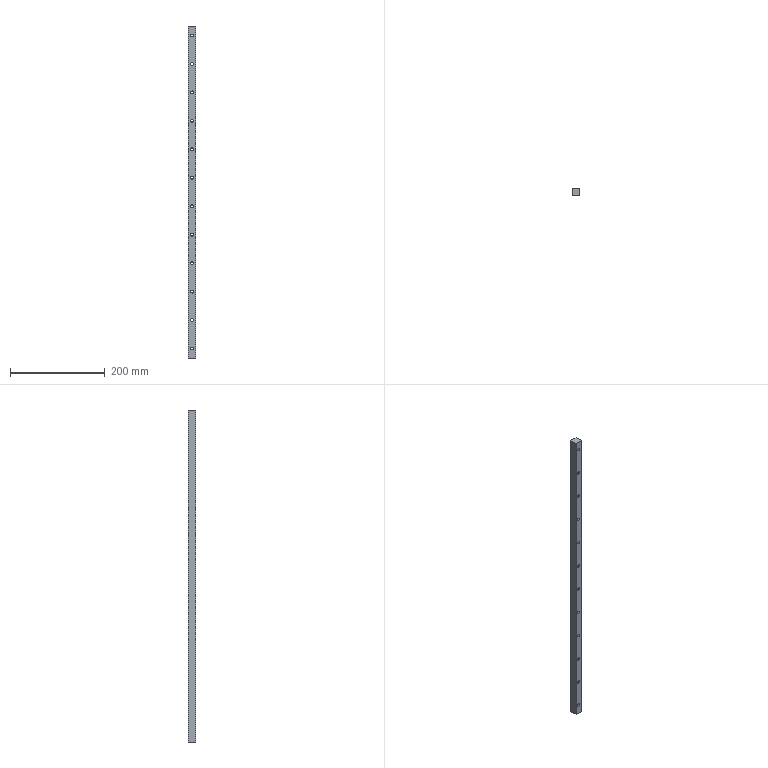Part | 1 solid | 30 faces | box 15 x 15 x 700 mm | volume 152411 mm3 | cylinder 24 | plane 6 | commonest cylinder face diameters 6 x24
STEP:
#1=CARTESIAN_POINT('',(7.5,0.,677.));
#2=VERTEX_POINT('',#1);
#3=CARTESIAN_POINT('',(7.5,0.,683.));
#4=VERTEX_POINT('',#3);
#5=CARTESIAN_POINT('',(7.5,0.,680.));
#6=DIRECTION('',(0.,1.,0.));
#7=DIRECTION('',(0.,0.,1.));
#8=AXIS2_PLACEMENT_3D('',#5,#6,#7);
#9=CIRCLE('',#8,3.);
#10=EDGE_CURVE('',#2,#4,#9,.T.);
#11=ORIENTED_EDGE('',*,*,#10,.F.);
#12=CARTESIAN_POINT('',(7.5,15.,677.));
#13=VERTEX_POINT('',#12);
#14=CARTESIAN_POINT('',(7.5,-35.,677.));
#15=DIRECTION('',(0.,1.,0.));
#16=VECTOR('',#15,1000.);
#17=LINE('',#14,#16);
#18=EDGE_CURVE('',#2,#13,#17,.T.);
#19=ORIENTED_EDGE('',*,*,#18,.T.);
#20=CARTESIAN_POINT('',(7.5,15.,683.));
#21=VERTEX_POINT('',#20);
#22=CARTESIAN_POINT('',(7.5,15.,680.));
#23=DIRECTION('',(0.,1.,0.));
#24=DIRECTION('',(0.,0.,1.));
#25=AXIS2_PLACEMENT_3D('',#22,#23,#24);
#26=CIRCLE('',#25,3.);
#27=EDGE_CURVE('',#13,#21,#26,.T.);
#28=ORIENTED_EDGE('',*,*,#27,.T.);
#29=CARTESIAN_POINT('',(7.5,-35.,683.));
#30=DIRECTION('',(0.,1.,0.));
#31=VECTOR('',#30,1000.);
#32=LINE('',#29,#31);
#33=EDGE_CURVE('',#4,#21,#32,.T.);
#34=ORIENTED_EDGE('',*,*,#33,.F.);
#35=EDGE_LOOP('',(#11,#19,#28,#34));
#36=FACE_OUTER_BOUND('',#35,.T.);
#37=CARTESIAN_POINT('',(7.5,-35.,680.));
#38=DIRECTION('',(0.,1.,0.));
#39=DIRECTION('',(0.,0.,1.));
#40=AXIS2_PLACEMENT_3D('',#37,#38,#39);
#41=CYLINDRICAL_SURFACE('',#40,3.);
#42=ADVANCED_FACE('',(#36),#41,.F.);
#43=CARTESIAN_POINT('',(7.5,0.,617.));
#44=VERTEX_POINT('',#43);
#45=CARTESIAN_POINT('',(7.5,0.,623.));
#46=VERTEX_POINT('',#45);
#47=CARTESIAN_POINT('',(7.5,0.,620.));
#48=DIRECTION('',(0.,1.,0.));
#49=DIRECTION('',(0.,0.,1.));
#50=AXIS2_PLACEMENT_3D('',#47,#48,#49);
#51=CIRCLE('',#50,3.);
#52=EDGE_CURVE('',#44,#46,#51,.T.);
#53=ORIENTED_EDGE('',*,*,#52,.F.);
#54=CARTESIAN_POINT('',(7.5,15.,617.));
#55=VERTEX_POINT('',#54);
#56=CARTESIAN_POINT('',(7.5,-35.,617.));
#57=DIRECTION('',(0.,1.,0.));
#58=VECTOR('',#57,1000.);
#59=LINE('',#56,#58);
#60=EDGE_CURVE('',#44,#55,#59,.T.);
#61=ORIENTED_EDGE('',*,*,#60,.T.);
#62=CARTESIAN_POINT('',(7.5,15.,623.));
#63=VERTEX_POINT('',#62);
#64=CARTESIAN_POINT('',(7.5,15.,620.));
#65=DIRECTION('',(0.,1.,0.));
#66=DIRECTION('',(0.,0.,1.));
#67=AXIS2_PLACEMENT_3D('',#64,#65,#66);
#68=CIRCLE('',#67,3.);
#69=EDGE_CURVE('',#55,#63,#68,.T.);
#70=ORIENTED_EDGE('',*,*,#69,.T.);
#71=CARTESIAN_POINT('',(7.5,-35.,623.));
#72=DIRECTION('',(0.,1.,0.));
#73=VECTOR('',#72,1000.);
#74=LINE('',#71,#73);
#75=EDGE_CURVE('',#46,#63,#74,.T.);
#76=ORIENTED_EDGE('',*,*,#75,.F.);
#77=EDGE_LOOP('',(#53,#61,#70,#76));
#78=FACE_OUTER_BOUND('',#77,.T.);
#79=CARTESIAN_POINT('',(7.5,-35.,620.));
#80=DIRECTION('',(0.,1.,0.));
#81=DIRECTION('',(0.,0.,1.));
#82=AXIS2_PLACEMENT_3D('',#79,#80,#81);
#83=CYLINDRICAL_SURFACE('',#82,3.);
#84=ADVANCED_FACE('',(#78),#83,.F.);
#85=CARTESIAN_POINT('',(7.5,0.,557.));
#86=VERTEX_POINT('',#85);
#87=CARTESIAN_POINT('',(7.5,0.,563.));
#88=VERTEX_POINT('',#87);
#89=CARTESIAN_POINT('',(7.5,0.,560.));
#90=DIRECTION('',(0.,1.,0.));
#91=DIRECTION('',(0.,0.,1.));
#92=AXIS2_PLACEMENT_3D('',#89,#90,#91);
#93=CIRCLE('',#92,3.);
#94=EDGE_CURVE('',#86,#88,#93,.T.);
#95=ORIENTED_EDGE('',*,*,#94,.F.);
#96=CARTESIAN_POINT('',(7.5,15.,557.));
#97=VERTEX_POINT('',#96);
#98=CARTESIAN_POINT('',(7.5,-35.,557.));
#99=DIRECTION('',(0.,1.,0.));
#100=VECTOR('',#99,1000.);
#101=LINE('',#98,#100);
#102=EDGE_CURVE('',#86,#97,#101,.T.);
#103=ORIENTED_EDGE('',*,*,#102,.T.);
#104=CARTESIAN_POINT('',(7.5,15.,563.));
#105=VERTEX_POINT('',#104);
#106=CARTESIAN_POINT('',(7.5,15.,560.));
#107=DIRECTION('',(0.,1.,0.));
#108=DIRECTION('',(0.,0.,1.));
#109=AXIS2_PLACEMENT_3D('',#106,#107,#108);
#110=CIRCLE('',#109,3.);
#111=EDGE_CURVE('',#97,#105,#110,.T.);
#112=ORIENTED_EDGE('',*,*,#111,.T.);
#113=CARTESIAN_POINT('',(7.5,-35.,563.));
#114=DIRECTION('',(0.,1.,0.));
#115=VECTOR('',#114,1000.);
#116=LINE('',#113,#115);
#117=EDGE_CURVE('',#88,#105,#116,.T.);
#118=ORIENTED_EDGE('',*,*,#117,.F.);
#119=EDGE_LOOP('',(#95,#103,#112,#118));
#120=FACE_OUTER_BOUND('',#119,.T.);
#121=CARTESIAN_POINT('',(7.5,-35.,560.));
#122=DIRECTION('',(0.,1.,0.));
#123=DIRECTION('',(0.,0.,1.));
#124=AXIS2_PLACEMENT_3D('',#121,#122,#123);
#125=CYLINDRICAL_SURFACE('',#124,3.);
#126=ADVANCED_FACE('',(#120),#125,.F.);
#127=CARTESIAN_POINT('',(7.5,0.,497.));
#128=VERTEX_POINT('',#127);
#129=CARTESIAN_POINT('',(7.5,0.,503.));
#130=VERTEX_POINT('',#129);
#131=CARTESIAN_POINT('',(7.5,0.,500.));
#132=DIRECTION('',(0.,1.,0.));
#133=DIRECTION('',(0.,0.,1.));
#134=AXIS2_PLACEMENT_3D('',#131,#132,#133);
#135=CIRCLE('',#134,3.);
#136=EDGE_CURVE('',#128,#130,#135,.T.);
#137=ORIENTED_EDGE('',*,*,#136,.F.);
#138=CARTESIAN_POINT('',(7.5,15.,497.));
#139=VERTEX_POINT('',#138);
#140=CARTESIAN_POINT('',(7.5,-35.,497.));
#141=DIRECTION('',(0.,1.,0.));
#142=VECTOR('',#141,1000.);
#143=LINE('',#140,#142);
#144=EDGE_CURVE('',#128,#139,#143,.T.);
#145=ORIENTED_EDGE('',*,*,#144,.T.);
#146=CARTESIAN_POINT('',(7.5,15.,503.));
#147=VERTEX_POINT('',#146);
#148=CARTESIAN_POINT('',(7.5,15.,500.));
#149=DIRECTION('',(0.,1.,0.));
#150=DIRECTION('',(0.,0.,1.));
#151=AXIS2_PLACEMENT_3D('',#148,#149,#150);
#152=CIRCLE('',#151,3.);
#153=EDGE_CURVE('',#139,#147,#152,.T.);
#154=ORIENTED_EDGE('',*,*,#153,.T.);
#155=CARTESIAN_POINT('',(7.5,-35.,503.));
#156=DIRECTION('',(0.,1.,0.));
#157=VECTOR('',#156,1000.);
#158=LINE('',#155,#157);
#159=EDGE_CURVE('',#130,#147,#158,.T.);
#160=ORIENTED_EDGE('',*,*,#159,.F.);
#161=EDGE_LOOP('',(#137,#145,#154,#160));
#162=FACE_OUTER_BOUND('',#161,.T.);
#163=CARTESIAN_POINT('',(7.5,-35.,500.));
#164=DIRECTION('',(0.,1.,0.));
#165=DIRECTION('',(0.,0.,1.));
#166=AXIS2_PLACEMENT_3D('',#163,#164,#165);
#167=CYLINDRICAL_SURFACE('',#166,3.);
#168=ADVANCED_FACE('',(#162),#167,.F.);
#169=CARTESIAN_POINT('',(7.5,0.,437.));
#170=VERTEX_POINT('',#169);
#171=CARTESIAN_POINT('',(7.5,0.,443.));
#172=VERTEX_POINT('',#171);
#173=CARTESIAN_POINT('',(7.5,0.,440.));
#174=DIRECTION('',(0.,1.,0.));
#175=DIRECTION('',(0.,0.,1.));
#176=AXIS2_PLACEMENT_3D('',#173,#174,#175);
#177=CIRCLE('',#176,3.);
#178=EDGE_CURVE('',#170,#172,#177,.T.);
#179=ORIENTED_EDGE('',*,*,#178,.F.);
#180=CARTESIAN_POINT('',(7.5,15.,437.));
#181=VERTEX_POINT('',#180);
#182=CARTESIAN_POINT('',(7.5,-35.,437.));
#183=DIRECTION('',(0.,1.,0.));
#184=VECTOR('',#183,1000.);
#185=LINE('',#182,#184);
#186=EDGE_CURVE('',#170,#181,#185,.T.);
#187=ORIENTED_EDGE('',*,*,#186,.T.);
#188=CARTESIAN_POINT('',(7.5,15.,443.));
#189=VERTEX_POINT('',#188);
#190=CARTESIAN_POINT('',(7.5,15.,440.));
#191=DIRECTION('',(0.,1.,0.));
#192=DIRECTION('',(0.,0.,1.));
#193=AXIS2_PLACEMENT_3D('',#190,#191,#192);
#194=CIRCLE('',#193,3.);
#195=EDGE_CURVE('',#181,#189,#194,.T.);
#196=ORIENTED_EDGE('',*,*,#195,.T.);
#197=CARTESIAN_POINT('',(7.5,-35.,443.));
#198=DIRECTION('',(0.,1.,0.));
#199=VECTOR('',#198,1000.);
#200=LINE('',#197,#199);
#201=EDGE_CURVE('',#172,#189,#200,.T.);
#202=ORIENTED_EDGE('',*,*,#201,.F.);
#203=EDGE_LOOP('',(#179,#187,#196,#202));
#204=FACE_OUTER_BOUND('',#203,.T.);
#205=CARTESIAN_POINT('',(7.5,-35.,440.));
#206=DIRECTION('',(0.,1.,0.));
#207=DIRECTION('',(0.,0.,1.));
#208=AXIS2_PLACEMENT_3D('',#205,#206,#207);
#209=CYLINDRICAL_SURFACE('',#208,3.);
#210=ADVANCED_FACE('',(#204),#209,.F.);
#211=CARTESIAN_POINT('',(7.5,0.,377.));
#212=VERTEX_POINT('',#211);
#213=CARTESIAN_POINT('',(7.5,0.,383.));
#214=VERTEX_POINT('',#213);
#215=CARTESIAN_POINT('',(7.5,0.,380.));
#216=DIRECTION('',(0.,1.,0.));
#217=DIRECTION('',(0.,0.,1.));
#218=AXIS2_PLACEMENT_3D('',#215,#216,#217);
#219=CIRCLE('',#218,3.);
#220=EDGE_CURVE('',#212,#214,#219,.T.);
#221=ORIENTED_EDGE('',*,*,#220,.F.);
#222=CARTESIAN_POINT('',(7.5,15.,377.));
#223=VERTEX_POINT('',#222);
#224=CARTESIAN_POINT('',(7.5,-35.,377.));
#225=DIRECTION('',(0.,1.,0.));
#226=VECTOR('',#225,1000.);
#227=LINE('',#224,#226);
#228=EDGE_CURVE('',#212,#223,#227,.T.);
#229=ORIENTED_EDGE('',*,*,#228,.T.);
#230=CARTESIAN_POINT('',(7.5,15.,383.));
#231=VERTEX_POINT('',#230);
#232=CARTESIAN_POINT('',(7.5,15.,380.));
#233=DIRECTION('',(0.,1.,0.));
#234=DIRECTION('',(0.,0.,1.));
#235=AXIS2_PLACEMENT_3D('',#232,#233,#234);
#236=CIRCLE('',#235,3.);
#237=EDGE_CURVE('',#223,#231,#236,.T.);
#238=ORIENTED_EDGE('',*,*,#237,.T.);
#239=CARTESIAN_POINT('',(7.5,-35.,383.));
#240=DIRECTION('',(0.,1.,0.));
#241=VECTOR('',#240,1000.);
#242=LINE('',#239,#241);
#243=EDGE_CURVE('',#214,#231,#242,.T.);
#244=ORIENTED_EDGE('',*,*,#243,.F.);
#245=EDGE_LOOP('',(#221,#229,#238,#244));
#246=FACE_OUTER_BOUND('',#245,.T.);
#247=CARTESIAN_POINT('',(7.5,-35.,380.));
#248=DIRECTION('',(0.,1.,0.));
#249=DIRECTION('',(0.,0.,1.));
#250=AXIS2_PLACEMENT_3D('',#247,#248,#249);
#251=CYLINDRICAL_SURFACE('',#250,3.);
#252=ADVANCED_FACE('',(#246),#251,.F.);
#253=CARTESIAN_POINT('',(7.5,0.,317.));
#254=VERTEX_POINT('',#253);
#255=CARTESIAN_POINT('',(7.5,0.,323.));
#256=VERTEX_POINT('',#255);
#257=CARTESIAN_POINT('',(7.5,0.,320.));
#258=DIRECTION('',(0.,1.,0.));
#259=DIRECTION('',(0.,0.,1.));
#260=AXIS2_PLACEMENT_3D('',#257,#258,#259);
#261=CIRCLE('',#260,3.);
#262=EDGE_CURVE('',#254,#256,#261,.T.);
#263=ORIENTED_EDGE('',*,*,#262,.F.);
#264=CARTESIAN_POINT('',(7.5,15.,317.));
#265=VERTEX_POINT('',#264);
#266=CARTESIAN_POINT('',(7.5,-35.,317.));
#267=DIRECTION('',(0.,1.,0.));
#268=VECTOR('',#267,1000.);
#269=LINE('',#266,#268);
#270=EDGE_CURVE('',#254,#265,#269,.T.);
#271=ORIENTED_EDGE('',*,*,#270,.T.);
#272=CARTESIAN_POINT('',(7.5,15.,323.));
#273=VERTEX_POINT('',#272);
#274=CARTESIAN_POINT('',(7.5,15.,320.));
#275=DIRECTION('',(0.,1.,0.));
#276=DIRECTION('',(0.,0.,1.));
#277=AXIS2_PLACEMENT_3D('',#274,#275,#276);
#278=CIRCLE('',#277,3.);
#279=EDGE_CURVE('',#265,#273,#278,.T.);
#280=ORIENTED_EDGE('',*,*,#279,.T.);
#281=CARTESIAN_POINT('',(7.5,-35.,323.));
#282=DIRECTION('',(0.,1.,0.));
#283=VECTOR('',#282,1000.);
#284=LINE('',#281,#283);
#285=EDGE_CURVE('',#256,#273,#284,.T.);
#286=ORIENTED_EDGE('',*,*,#285,.F.);
#287=EDGE_LOOP('',(#263,#271,#280,#286));
#288=FACE_OUTER_BOUND('',#287,.T.);
#289=CARTESIAN_POINT('',(7.5,-35.,320.));
#290=DIRECTION('',(0.,1.,0.));
#291=DIRECTION('',(0.,0.,1.));
#292=AXIS2_PLACEMENT_3D('',#289,#290,#291);
#293=CYLINDRICAL_SURFACE('',#292,3.);
#294=ADVANCED_FACE('',(#288),#293,.F.);
#295=CARTESIAN_POINT('',(7.5,0.,257.));
#296=VERTEX_POINT('',#295);
#297=CARTESIAN_POINT('',(7.5,0.,263.));
#298=VERTEX_POINT('',#297);
#299=CARTESIAN_POINT('',(7.5,0.,260.));
#300=DIRECTION('',(0.,1.,0.));
#301=DIRECTION('',(0.,0.,1.));
#302=AXIS2_PLACEMENT_3D('',#299,#300,#301);
#303=CIRCLE('',#302,3.);
#304=EDGE_CURVE('',#296,#298,#303,.T.);
#305=ORIENTED_EDGE('',*,*,#304,.F.);
#306=CARTESIAN_POINT('',(7.5,15.,257.));
#307=VERTEX_POINT('',#306);
#308=CARTESIAN_POINT('',(7.5,-35.,257.));
#309=DIRECTION('',(0.,1.,0.));
#310=VECTOR('',#309,1000.);
#311=LINE('',#308,#310);
#312=EDGE_CURVE('',#296,#307,#311,.T.);
#313=ORIENTED_EDGE('',*,*,#312,.T.);
#314=CARTESIAN_POINT('',(7.5,15.,263.));
#315=VERTEX_POINT('',#314);
#316=CARTESIAN_POINT('',(7.5,15.,260.));
#317=DIRECTION('',(0.,1.,0.));
#318=DIRECTION('',(0.,0.,1.));
#319=AXIS2_PLACEMENT_3D('',#316,#317,#318);
#320=CIRCLE('',#319,3.);
#321=EDGE_CURVE('',#307,#315,#320,.T.);
#322=ORIENTED_EDGE('',*,*,#321,.T.);
#323=CARTESIAN_POINT('',(7.5,-35.,263.));
#324=DIRECTION('',(0.,1.,0.));
#325=VECTOR('',#324,1000.);
#326=LINE('',#323,#325);
#327=EDGE_CURVE('',#298,#315,#326,.T.);
#328=ORIENTED_EDGE('',*,*,#327,.F.);
#329=EDGE_LOOP('',(#305,#313,#322,#328));
#330=FACE_OUTER_BOUND('',#329,.T.);
#331=CARTESIAN_POINT('',(7.5,-35.,260.));
#332=DIRECTION('',(0.,1.,0.));
#333=DIRECTION('',(0.,0.,1.));
#334=AXIS2_PLACEMENT_3D('',#331,#332,#333);
#335=CYLINDRICAL_SURFACE('',#334,3.);
#336=ADVANCED_FACE('',(#330),#335,.F.);
#337=CARTESIAN_POINT('',(7.5,0.,197.));
#338=VERTEX_POINT('',#337);
#339=CARTESIAN_POINT('',(7.5,0.,203.));
#340=VERTEX_POINT('',#339);
#341=CARTESIAN_POINT('',(7.5,0.,200.));
#342=DIRECTION('',(0.,1.,0.));
#343=DIRECTION('',(0.,0.,1.));
#344=AXIS2_PLACEMENT_3D('',#341,#342,#343);
#345=CIRCLE('',#344,3.);
#346=EDGE_CURVE('',#338,#340,#345,.T.);
#347=ORIENTED_EDGE('',*,*,#346,.F.);
#348=CARTESIAN_POINT('',(7.5,15.,197.));
#349=VERTEX_POINT('',#348);
#350=CARTESIAN_POINT('',(7.5,-35.,197.));
#351=DIRECTION('',(0.,1.,0.));
#352=VECTOR('',#351,1000.);
#353=LINE('',#350,#352);
#354=EDGE_CURVE('',#338,#349,#353,.T.);
#355=ORIENTED_EDGE('',*,*,#354,.T.);
#356=CARTESIAN_POINT('',(7.5,15.,203.));
#357=VERTEX_POINT('',#356);
#358=CARTESIAN_POINT('',(7.5,15.,200.));
#359=DIRECTION('',(0.,1.,0.));
#360=DIRECTION('',(0.,0.,1.));
#361=AXIS2_PLACEMENT_3D('',#358,#359,#360);
#362=CIRCLE('',#361,3.);
#363=EDGE_CURVE('',#349,#357,#362,.T.);
#364=ORIENTED_EDGE('',*,*,#363,.T.);
#365=CARTESIAN_POINT('',(7.5,-35.,203.));
#366=DIRECTION('',(0.,1.,0.));
#367=VECTOR('',#366,1000.);
#368=LINE('',#365,#367);
#369=EDGE_CURVE('',#340,#357,#368,.T.);
#370=ORIENTED_EDGE('',*,*,#369,.F.);
#371=EDGE_LOOP('',(#347,#355,#364,#370));
#372=FACE_OUTER_BOUND('',#371,.T.);
#373=CARTESIAN_POINT('',(7.5,-35.,200.));
#374=DIRECTION('',(0.,1.,0.));
#375=DIRECTION('',(0.,0.,1.));
#376=AXIS2_PLACEMENT_3D('',#373,#374,#375);
#377=CYLINDRICAL_SURFACE('',#376,3.);
#378=ADVANCED_FACE('',(#372),#377,.F.);
#379=CARTESIAN_POINT('',(7.5,0.,137.));
#380=VERTEX_POINT('',#379);
#381=CARTESIAN_POINT('',(7.5,0.,143.));
#382=VERTEX_POINT('',#381);
#383=CARTESIAN_POINT('',(7.5,0.,140.));
#384=DIRECTION('',(0.,1.,0.));
#385=DIRECTION('',(0.,0.,1.));
#386=AXIS2_PLACEMENT_3D('',#383,#384,#385);
#387=CIRCLE('',#386,3.);
#388=EDGE_CURVE('',#380,#382,#387,.T.);
#389=ORIENTED_EDGE('',*,*,#388,.F.);
#390=CARTESIAN_POINT('',(7.5,15.,137.));
#391=VERTEX_POINT('',#390);
#392=CARTESIAN_POINT('',(7.5,-35.,137.));
#393=DIRECTION('',(0.,1.,0.));
#394=VECTOR('',#393,1000.);
#395=LINE('',#392,#394);
#396=EDGE_CURVE('',#380,#391,#395,.T.);
#397=ORIENTED_EDGE('',*,*,#396,.T.);
#398=CARTESIAN_POINT('',(7.5,15.,143.));
#399=VERTEX_POINT('',#398);
#400=CARTESIAN_POINT('',(7.5,15.,140.));
#401=DIRECTION('',(0.,1.,0.));
#402=DIRECTION('',(0.,0.,1.));
#403=AXIS2_PLACEMENT_3D('',#400,#401,#402);
#404=CIRCLE('',#403,3.);
#405=EDGE_CURVE('',#391,#399,#404,.T.);
#406=ORIENTED_EDGE('',*,*,#405,.T.);
#407=CARTESIAN_POINT('',(7.5,-35.,143.));
#408=DIRECTION('',(0.,1.,0.));
#409=VECTOR('',#408,1000.);
#410=LINE('',#407,#409);
#411=EDGE_CURVE('',#382,#399,#410,.T.);
#412=ORIENTED_EDGE('',*,*,#411,.F.);
#413=EDGE_LOOP('',(#389,#397,#406,#412));
#414=FACE_OUTER_BOUND('',#413,.T.);
#415=CARTESIAN_POINT('',(7.5,-35.,140.));
#416=DIRECTION('',(0.,1.,0.));
#417=DIRECTION('',(0.,0.,1.));
#418=AXIS2_PLACEMENT_3D('',#415,#416,#417);
#419=CYLINDRICAL_SURFACE('',#418,3.);
#420=ADVANCED_FACE('',(#414),#419,.F.);
#421=CARTESIAN_POINT('',(7.5,0.,77.));
#422=VERTEX_POINT('',#421);
#423=CARTESIAN_POINT('',(7.5,0.,83.));
#424=VERTEX_POINT('',#423);
#425=CARTESIAN_POINT('',(7.5,0.,80.));
#426=DIRECTION('',(0.,1.,0.));
#427=DIRECTION('',(0.,0.,1.));
#428=AXIS2_PLACEMENT_3D('',#425,#426,#427);
#429=CIRCLE('',#428,3.);
#430=EDGE_CURVE('',#422,#424,#429,.T.);
#431=ORIENTED_EDGE('',*,*,#430,.F.);
#432=CARTESIAN_POINT('',(7.5,15.,77.));
#433=VERTEX_POINT('',#432);
#434=CARTESIAN_POINT('',(7.5,-35.,77.));
#435=DIRECTION('',(0.,1.,0.));
#436=VECTOR('',#435,1000.);
#437=LINE('',#434,#436);
#438=EDGE_CURVE('',#422,#433,#437,.T.);
#439=ORIENTED_EDGE('',*,*,#438,.T.);
#440=CARTESIAN_POINT('',(7.5,15.,83.));
#441=VERTEX_POINT('',#440);
#442=CARTESIAN_POINT('',(7.5,15.,80.));
#443=DIRECTION('',(0.,1.,0.));
#444=DIRECTION('',(0.,0.,1.));
#445=AXIS2_PLACEMENT_3D('',#442,#443,#444);
#446=CIRCLE('',#445,3.);
#447=EDGE_CURVE('',#433,#441,#446,.T.);
#448=ORIENTED_EDGE('',*,*,#447,.T.);
#449=CARTESIAN_POINT('',(7.5,-35.,83.));
#450=DIRECTION('',(0.,1.,0.));
#451=VECTOR('',#450,1000.);
#452=LINE('',#449,#451);
#453=EDGE_CURVE('',#424,#441,#452,.T.);
#454=ORIENTED_EDGE('',*,*,#453,.F.);
#455=EDGE_LOOP('',(#431,#439,#448,#454));
#456=FACE_OUTER_BOUND('',#455,.T.);
#457=CARTESIAN_POINT('',(7.5,-35.,80.));
#458=DIRECTION('',(0.,1.,0.));
#459=DIRECTION('',(0.,0.,1.));
#460=AXIS2_PLACEMENT_3D('',#457,#458,#459);
#461=CYLINDRICAL_SURFACE('',#460,3.);
#462=ADVANCED_FACE('',(#456),#461,.F.);
#463=CARTESIAN_POINT('',(7.5,0.,17.));
#464=VERTEX_POINT('',#463);
#465=CARTESIAN_POINT('',(7.5,0.,23.));
#466=VERTEX_POINT('',#465);
#467=CARTESIAN_POINT('',(7.5,0.,20.));
#468=DIRECTION('',(0.,1.,0.));
#469=DIRECTION('',(0.,0.,1.));
#470=AXIS2_PLACEMENT_3D('',#467,#468,#469);
#471=CIRCLE('',#470,3.);
#472=EDGE_CURVE('',#464,#466,#471,.T.);
#473=ORIENTED_EDGE('',*,*,#472,.F.);
#474=CARTESIAN_POINT('',(7.5,15.,17.));
#475=VERTEX_POINT('',#474);
#476=CARTESIAN_POINT('',(7.5,-35.,17.));
#477=DIRECTION('',(0.,1.,0.));
#478=VECTOR('',#477,1000.);
#479=LINE('',#476,#478);
#480=EDGE_CURVE('',#464,#475,#479,.T.);
#481=ORIENTED_EDGE('',*,*,#480,.T.);
#482=CARTESIAN_POINT('',(7.5,15.,23.));
#483=VERTEX_POINT('',#482);
#484=CARTESIAN_POINT('',(7.5,15.,20.));
#485=DIRECTION('',(0.,1.,0.));
#486=DIRECTION('',(0.,0.,1.));
#487=AXIS2_PLACEMENT_3D('',#484,#485,#486);
#488=CIRCLE('',#487,3.);
#489=EDGE_CURVE('',#475,#483,#488,.T.);
#490=ORIENTED_EDGE('',*,*,#489,.T.);
#491=CARTESIAN_POINT('',(7.5,-35.,23.));
#492=DIRECTION('',(0.,1.,0.));
#493=VECTOR('',#492,1000.);
#494=LINE('',#491,#493);
#495=EDGE_CURVE('',#466,#483,#494,.T.);
#496=ORIENTED_EDGE('',*,*,#495,.F.);
#497=EDGE_LOOP('',(#473,#481,#490,#496));
#498=FACE_OUTER_BOUND('',#497,.T.);
#499=CARTESIAN_POINT('',(7.5,-35.,20.));
#500=DIRECTION('',(0.,1.,0.));
#501=DIRECTION('',(0.,0.,1.));
#502=AXIS2_PLACEMENT_3D('',#499,#500,#501);
#503=CYLINDRICAL_SURFACE('',#502,3.);
#504=ADVANCED_FACE('',(#498),#503,.F.);
#505=CARTESIAN_POINT('',(0.,15.,0.));
#506=VERTEX_POINT('',#505);
#507=CARTESIAN_POINT('',(0.,0.,0.));
#508=VERTEX_POINT('',#507);
#509=CARTESIAN_POINT('',(0.,0.,0.));
#510=DIRECTION('',(0.,-1.,0.));
#511=VECTOR('',#510,1000.);
#512=LINE('',#509,#511);
#513=EDGE_CURVE('',#506,#508,#512,.T.);
#514=ORIENTED_EDGE('',*,*,#513,.T.);
#515=CARTESIAN_POINT('',(0.,0.,700.));
#516=VERTEX_POINT('',#515);
#517=CARTESIAN_POINT('',(0.,0.,700.));
#518=DIRECTION('',(0.,0.,-1.));
#519=VECTOR('',#518,1000.);
#520=LINE('',#517,#519);
#521=EDGE_CURVE('',#516,#508,#520,.T.);
#522=ORIENTED_EDGE('',*,*,#521,.F.);
#523=CARTESIAN_POINT('',(0.,15.,700.));
#524=VERTEX_POINT('',#523);
#525=CARTESIAN_POINT('',(0.,0.,700.));
#526=DIRECTION('',(0.,-1.,0.));
#527=VECTOR('',#526,1000.);
#528=LINE('',#525,#527);
#529=EDGE_CURVE('',#524,#516,#528,.T.);
#530=ORIENTED_EDGE('',*,*,#529,.F.);
#531=CARTESIAN_POINT('',(0.,15.,700.));
#532=DIRECTION('',(0.,0.,-1.));
#533=VECTOR('',#532,1000.);
#534=LINE('',#531,#533);
#535=EDGE_CURVE('',#524,#506,#534,.T.);
#536=ORIENTED_EDGE('',*,*,#535,.T.);
#537=EDGE_LOOP('',(#514,#522,#530,#536));
#538=FACE_OUTER_BOUND('',#537,.T.);
#539=CARTESIAN_POINT('',(0.,0.,700.));
#540=DIRECTION('',(1.,0.,0.));
#541=DIRECTION('',(0.,0.,-1.));
#542=AXIS2_PLACEMENT_3D('',#539,#540,#541);
#543=PLANE('',#542);
#544=ADVANCED_FACE('',(#538),#543,.F.);
#545=CARTESIAN_POINT('',(7.5,0.,80.));
#546=DIRECTION('',(0.,1.,0.));
#547=DIRECTION('',(0.,0.,1.));
#548=AXIS2_PLACEMENT_3D('',#545,#546,#547);
#549=CIRCLE('',#548,3.);
#550=EDGE_CURVE('',#424,#422,#549,.T.);
#551=ORIENTED_EDGE('',*,*,#550,.T.);
#552=ORIENTED_EDGE('',*,*,#430,.T.);
#553=EDGE_LOOP('',(#551,#552));
#554=FACE_BOUND('',#553,.T.);
#555=CARTESIAN_POINT('',(7.5,0.,20.));
#556=DIRECTION('',(0.,1.,0.));
#557=DIRECTION('',(0.,0.,1.));
#558=AXIS2_PLACEMENT_3D('',#555,#556,#557);
#559=CIRCLE('',#558,3.);
#560=EDGE_CURVE('',#466,#464,#559,.T.);
#561=ORIENTED_EDGE('',*,*,#560,.T.);
#562=ORIENTED_EDGE('',*,*,#472,.T.);
#563=EDGE_LOOP('',(#561,#562));
#564=FACE_BOUND('',#563,.T.);
#565=CARTESIAN_POINT('',(15.,0.,0.));
#566=VERTEX_POINT('',#565);
#567=CARTESIAN_POINT('',(0.,0.,0.));
#568=DIRECTION('',(1.,0.,0.));
#569=VECTOR('',#568,1000.);
#570=LINE('',#567,#569);
#571=EDGE_CURVE('',#508,#566,#570,.T.);
#572=ORIENTED_EDGE('',*,*,#571,.T.);
#573=CARTESIAN_POINT('',(15.,0.,700.));
#574=VERTEX_POINT('',#573);
#575=CARTESIAN_POINT('',(15.,0.,700.));
#576=DIRECTION('',(0.,0.,-1.));
#577=VECTOR('',#576,1000.);
#578=LINE('',#575,#577);
#579=EDGE_CURVE('',#574,#566,#578,.T.);
#580=ORIENTED_EDGE('',*,*,#579,.F.);
#581=CARTESIAN_POINT('',(0.,0.,700.));
#582=DIRECTION('',(1.,0.,0.));
#583=VECTOR('',#582,1000.);
#584=LINE('',#581,#583);
#585=EDGE_CURVE('',#516,#574,#584,.T.);
#586=ORIENTED_EDGE('',*,*,#585,.F.);
#587=ORIENTED_EDGE('',*,*,#521,.T.);
#588=EDGE_LOOP('',(#572,#580,#586,#587));
#589=FACE_OUTER_BOUND('',#588,.T.);
#590=CARTESIAN_POINT('',(7.5,0.,140.));
#591=DIRECTION('',(0.,1.,0.));
#592=DIRECTION('',(0.,0.,1.));
#593=AXIS2_PLACEMENT_3D('',#590,#591,#592);
#594=CIRCLE('',#593,3.);
#595=EDGE_CURVE('',#382,#380,#594,.T.);
#596=ORIENTED_EDGE('',*,*,#595,.T.);
#597=ORIENTED_EDGE('',*,*,#388,.T.);
#598=EDGE_LOOP('',(#596,#597));
#599=FACE_BOUND('',#598,.T.);
#600=CARTESIAN_POINT('',(7.5,0.,200.));
#601=DIRECTION('',(0.,1.,0.));
#602=DIRECTION('',(0.,0.,1.));
#603=AXIS2_PLACEMENT_3D('',#600,#601,#602);
#604=CIRCLE('',#603,3.);
#605=EDGE_CURVE('',#340,#338,#604,.T.);
#606=ORIENTED_EDGE('',*,*,#605,.T.);
#607=ORIENTED_EDGE('',*,*,#346,.T.);
#608=EDGE_LOOP('',(#606,#607));
#609=FACE_BOUND('',#608,.T.);
#610=CARTESIAN_POINT('',(7.5,0.,260.));
#611=DIRECTION('',(0.,1.,0.));
#612=DIRECTION('',(0.,0.,1.));
#613=AXIS2_PLACEMENT_3D('',#610,#611,#612);
#614=CIRCLE('',#613,3.);
#615=EDGE_CURVE('',#298,#296,#614,.T.);
#616=ORIENTED_EDGE('',*,*,#615,.T.);
#617=ORIENTED_EDGE('',*,*,#304,.T.);
#618=EDGE_LOOP('',(#616,#617));
#619=FACE_BOUND('',#618,.T.);
#620=CARTESIAN_POINT('',(7.5,0.,320.));
#621=DIRECTION('',(0.,1.,0.));
#622=DIRECTION('',(0.,0.,1.));
#623=AXIS2_PLACEMENT_3D('',#620,#621,#622);
#624=CIRCLE('',#623,3.);
#625=EDGE_CURVE('',#256,#254,#624,.T.);
#626=ORIENTED_EDGE('',*,*,#625,.T.);
#627=ORIENTED_EDGE('',*,*,#262,.T.);
#628=EDGE_LOOP('',(#626,#627));
#629=FACE_BOUND('',#628,.T.);
#630=CARTESIAN_POINT('',(7.5,0.,380.));
#631=DIRECTION('',(0.,1.,0.));
#632=DIRECTION('',(0.,0.,1.));
#633=AXIS2_PLACEMENT_3D('',#630,#631,#632);
#634=CIRCLE('',#633,3.);
#635=EDGE_CURVE('',#214,#212,#634,.T.);
#636=ORIENTED_EDGE('',*,*,#635,.T.);
#637=ORIENTED_EDGE('',*,*,#220,.T.);
#638=EDGE_LOOP('',(#636,#637));
#639=FACE_BOUND('',#638,.T.);
#640=CARTESIAN_POINT('',(7.5,0.,440.));
#641=DIRECTION('',(0.,1.,0.));
#642=DIRECTION('',(0.,0.,1.));
#643=AXIS2_PLACEMENT_3D('',#640,#641,#642);
#644=CIRCLE('',#643,3.);
#645=EDGE_CURVE('',#172,#170,#644,.T.);
#646=ORIENTED_EDGE('',*,*,#645,.T.);
#647=ORIENTED_EDGE('',*,*,#178,.T.);
#648=EDGE_LOOP('',(#646,#647));
#649=FACE_BOUND('',#648,.T.);
#650=CARTESIAN_POINT('',(7.5,0.,500.));
#651=DIRECTION('',(0.,1.,0.));
#652=DIRECTION('',(0.,0.,1.));
#653=AXIS2_PLACEMENT_3D('',#650,#651,#652);
#654=CIRCLE('',#653,3.);
#655=EDGE_CURVE('',#130,#128,#654,.T.);
#656=ORIENTED_EDGE('',*,*,#655,.T.);
#657=ORIENTED_EDGE('',*,*,#136,.T.);
#658=EDGE_LOOP('',(#656,#657));
#659=FACE_BOUND('',#658,.T.);
#660=CARTESIAN_POINT('',(7.5,0.,560.));
#661=DIRECTION('',(0.,1.,0.));
#662=DIRECTION('',(0.,0.,1.));
#663=AXIS2_PLACEMENT_3D('',#660,#661,#662);
#664=CIRCLE('',#663,3.);
#665=EDGE_CURVE('',#88,#86,#664,.T.);
#666=ORIENTED_EDGE('',*,*,#665,.T.);
#667=ORIENTED_EDGE('',*,*,#94,.T.);
#668=EDGE_LOOP('',(#666,#667));
#669=FACE_BOUND('',#668,.T.);
#670=CARTESIAN_POINT('',(7.5,0.,620.));
#671=DIRECTION('',(0.,1.,0.));
#672=DIRECTION('',(0.,0.,1.));
#673=AXIS2_PLACEMENT_3D('',#670,#671,#672);
#674=CIRCLE('',#673,3.);
#675=EDGE_CURVE('',#46,#44,#674,.T.);
#676=ORIENTED_EDGE('',*,*,#675,.T.);
#677=ORIENTED_EDGE('',*,*,#52,.T.);
#678=EDGE_LOOP('',(#676,#677));
#679=FACE_BOUND('',#678,.T.);
#680=CARTESIAN_POINT('',(7.5,0.,680.));
#681=DIRECTION('',(0.,1.,0.));
#682=DIRECTION('',(0.,0.,1.));
#683=AXIS2_PLACEMENT_3D('',#680,#681,#682);
#684=CIRCLE('',#683,3.);
#685=EDGE_CURVE('',#4,#2,#684,.T.);
#686=ORIENTED_EDGE('',*,*,#685,.T.);
#687=ORIENTED_EDGE('',*,*,#10,.T.);
#688=EDGE_LOOP('',(#686,#687));
#689=FACE_BOUND('',#688,.T.);
#690=CARTESIAN_POINT('',(0.,0.,700.));
#691=DIRECTION('',(0.,1.,0.));
#692=DIRECTION('',(0.,0.,1.));
#693=AXIS2_PLACEMENT_3D('',#690,#691,#692);
#694=PLANE('',#693);
#695=ADVANCED_FACE('',(#554,#564,#589,#599,#609,#619,#629,#639,#649,#659,#669,#679,#689),#694,.F.);
#696=CARTESIAN_POINT('',(15.,15.,0.));
#697=VERTEX_POINT('',#696);
#698=CARTESIAN_POINT('',(15.,0.,0.));
#699=DIRECTION('',(0.,1.,0.));
#700=VECTOR('',#699,1000.);
#701=LINE('',#698,#700);
#702=EDGE_CURVE('',#566,#697,#701,.T.);
#703=ORIENTED_EDGE('',*,*,#702,.T.);
#704=CARTESIAN_POINT('',(15.,15.,700.));
#705=VERTEX_POINT('',#704);
#706=CARTESIAN_POINT('',(15.,15.,700.));
#707=DIRECTION('',(0.,0.,-1.));
#708=VECTOR('',#707,1000.);
#709=LINE('',#706,#708);
#710=EDGE_CURVE('',#705,#697,#709,.T.);
#711=ORIENTED_EDGE('',*,*,#710,.F.);
#712=CARTESIAN_POINT('',(15.,0.,700.));
#713=DIRECTION('',(0.,1.,0.));
#714=VECTOR('',#713,1000.);
#715=LINE('',#712,#714);
#716=EDGE_CURVE('',#574,#705,#715,.T.);
#717=ORIENTED_EDGE('',*,*,#716,.F.);
#718=ORIENTED_EDGE('',*,*,#579,.T.);
#719=EDGE_LOOP('',(#703,#711,#717,#718));
#720=FACE_OUTER_BOUND('',#719,.T.);
#721=CARTESIAN_POINT('',(15.,0.,700.));
#722=DIRECTION('',(-1.,0.,0.));
#723=DIRECTION('',(0.,0.,1.));
#724=AXIS2_PLACEMENT_3D('',#721,#722,#723);
#725=PLANE('',#724);
#726=ADVANCED_FACE('',(#720),#725,.F.);
#727=CARTESIAN_POINT('',(7.5,15.,80.));
#728=DIRECTION('',(0.,1.,0.));
#729=DIRECTION('',(0.,0.,1.));
#730=AXIS2_PLACEMENT_3D('',#727,#728,#729);
#731=CIRCLE('',#730,3.);
#732=EDGE_CURVE('',#441,#433,#731,.T.);
#733=ORIENTED_EDGE('',*,*,#732,.F.);
#734=ORIENTED_EDGE('',*,*,#447,.F.);
#735=EDGE_LOOP('',(#733,#734));
#736=FACE_BOUND('',#735,.T.);
#737=CARTESIAN_POINT('',(7.5,15.,20.));
#738=DIRECTION('',(0.,1.,0.));
#739=DIRECTION('',(0.,0.,1.));
#740=AXIS2_PLACEMENT_3D('',#737,#738,#739);
#741=CIRCLE('',#740,3.);
#742=EDGE_CURVE('',#483,#475,#741,.T.);
#743=ORIENTED_EDGE('',*,*,#742,.F.);
#744=ORIENTED_EDGE('',*,*,#489,.F.);
#745=EDGE_LOOP('',(#743,#744));
#746=FACE_BOUND('',#745,.T.);
#747=CARTESIAN_POINT('',(0.,15.,0.));
#748=DIRECTION('',(-1.,0.,0.));
#749=VECTOR('',#748,1000.);
#750=LINE('',#747,#749);
#751=EDGE_CURVE('',#697,#506,#750,.T.);
#752=ORIENTED_EDGE('',*,*,#751,.T.);
#753=ORIENTED_EDGE('',*,*,#535,.F.);
#754=CARTESIAN_POINT('',(0.,15.,700.));
#755=DIRECTION('',(-1.,0.,0.));
#756=VECTOR('',#755,1000.);
#757=LINE('',#754,#756);
#758=EDGE_CURVE('',#705,#524,#757,.T.);
#759=ORIENTED_EDGE('',*,*,#758,.F.);
#760=ORIENTED_EDGE('',*,*,#710,.T.);
#761=EDGE_LOOP('',(#752,#753,#759,#760));
#762=FACE_OUTER_BOUND('',#761,.T.);
#763=CARTESIAN_POINT('',(7.5,15.,140.));
#764=DIRECTION('',(0.,1.,0.));
#765=DIRECTION('',(0.,0.,1.));
#766=AXIS2_PLACEMENT_3D('',#763,#764,#765);
#767=CIRCLE('',#766,3.);
#768=EDGE_CURVE('',#399,#391,#767,.T.);
#769=ORIENTED_EDGE('',*,*,#768,.F.);
#770=ORIENTED_EDGE('',*,*,#405,.F.);
#771=EDGE_LOOP('',(#769,#770));
#772=FACE_BOUND('',#771,.T.);
#773=CARTESIAN_POINT('',(7.5,15.,200.));
#774=DIRECTION('',(0.,1.,0.));
#775=DIRECTION('',(0.,0.,1.));
#776=AXIS2_PLACEMENT_3D('',#773,#774,#775);
#777=CIRCLE('',#776,3.);
#778=EDGE_CURVE('',#357,#349,#777,.T.);
#779=ORIENTED_EDGE('',*,*,#778,.F.);
#780=ORIENTED_EDGE('',*,*,#363,.F.);
#781=EDGE_LOOP('',(#779,#780));
#782=FACE_BOUND('',#781,.T.);
#783=CARTESIAN_POINT('',(7.5,15.,260.));
#784=DIRECTION('',(0.,1.,0.));
#785=DIRECTION('',(0.,0.,1.));
#786=AXIS2_PLACEMENT_3D('',#783,#784,#785);
#787=CIRCLE('',#786,3.);
#788=EDGE_CURVE('',#315,#307,#787,.T.);
#789=ORIENTED_EDGE('',*,*,#788,.F.);
#790=ORIENTED_EDGE('',*,*,#321,.F.);
#791=EDGE_LOOP('',(#789,#790));
#792=FACE_BOUND('',#791,.T.);
#793=CARTESIAN_POINT('',(7.5,15.,320.));
#794=DIRECTION('',(0.,1.,0.));
#795=DIRECTION('',(0.,0.,1.));
#796=AXIS2_PLACEMENT_3D('',#793,#794,#795);
#797=CIRCLE('',#796,3.);
#798=EDGE_CURVE('',#273,#265,#797,.T.);
#799=ORIENTED_EDGE('',*,*,#798,.F.);
#800=ORIENTED_EDGE('',*,*,#279,.F.);
#801=EDGE_LOOP('',(#799,#800));
#802=FACE_BOUND('',#801,.T.);
#803=CARTESIAN_POINT('',(7.5,15.,380.));
#804=DIRECTION('',(0.,1.,0.));
#805=DIRECTION('',(0.,0.,1.));
#806=AXIS2_PLACEMENT_3D('',#803,#804,#805);
#807=CIRCLE('',#806,3.);
#808=EDGE_CURVE('',#231,#223,#807,.T.);
#809=ORIENTED_EDGE('',*,*,#808,.F.);
#810=ORIENTED_EDGE('',*,*,#237,.F.);
#811=EDGE_LOOP('',(#809,#810));
#812=FACE_BOUND('',#811,.T.);
#813=CARTESIAN_POINT('',(7.5,15.,440.));
#814=DIRECTION('',(0.,1.,0.));
#815=DIRECTION('',(0.,0.,1.));
#816=AXIS2_PLACEMENT_3D('',#813,#814,#815);
#817=CIRCLE('',#816,3.);
#818=EDGE_CURVE('',#189,#181,#817,.T.);
#819=ORIENTED_EDGE('',*,*,#818,.F.);
#820=ORIENTED_EDGE('',*,*,#195,.F.);
#821=EDGE_LOOP('',(#819,#820));
#822=FACE_BOUND('',#821,.T.);
#823=CARTESIAN_POINT('',(7.5,15.,500.));
#824=DIRECTION('',(0.,1.,0.));
#825=DIRECTION('',(0.,0.,1.));
#826=AXIS2_PLACEMENT_3D('',#823,#824,#825);
#827=CIRCLE('',#826,3.);
#828=EDGE_CURVE('',#147,#139,#827,.T.);
#829=ORIENTED_EDGE('',*,*,#828,.F.);
#830=ORIENTED_EDGE('',*,*,#153,.F.);
#831=EDGE_LOOP('',(#829,#830));
#832=FACE_BOUND('',#831,.T.);
#833=CARTESIAN_POINT('',(7.5,15.,560.));
#834=DIRECTION('',(0.,1.,0.));
#835=DIRECTION('',(0.,0.,1.));
#836=AXIS2_PLACEMENT_3D('',#833,#834,#835);
#837=CIRCLE('',#836,3.);
#838=EDGE_CURVE('',#105,#97,#837,.T.);
#839=ORIENTED_EDGE('',*,*,#838,.F.);
#840=ORIENTED_EDGE('',*,*,#111,.F.);
#841=EDGE_LOOP('',(#839,#840));
#842=FACE_BOUND('',#841,.T.);
#843=CARTESIAN_POINT('',(7.5,15.,620.));
#844=DIRECTION('',(0.,1.,0.));
#845=DIRECTION('',(0.,0.,1.));
#846=AXIS2_PLACEMENT_3D('',#843,#844,#845);
#847=CIRCLE('',#846,3.);
#848=EDGE_CURVE('',#63,#55,#847,.T.);
#849=ORIENTED_EDGE('',*,*,#848,.F.);
#850=ORIENTED_EDGE('',*,*,#69,.F.);
#851=EDGE_LOOP('',(#849,#850));
#852=FACE_BOUND('',#851,.T.);
#853=CARTESIAN_POINT('',(7.5,15.,680.));
#854=DIRECTION('',(0.,1.,0.));
#855=DIRECTION('',(0.,0.,1.));
#856=AXIS2_PLACEMENT_3D('',#853,#854,#855);
#857=CIRCLE('',#856,3.);
#858=EDGE_CURVE('',#21,#13,#857,.T.);
#859=ORIENTED_EDGE('',*,*,#858,.F.);
#860=ORIENTED_EDGE('',*,*,#27,.F.);
#861=EDGE_LOOP('',(#859,#860));
#862=FACE_BOUND('',#861,.T.);
#863=CARTESIAN_POINT('',(0.,15.,700.));
#864=DIRECTION('',(0.,-1.,0.));
#865=DIRECTION('',(0.,0.,-1.));
#866=AXIS2_PLACEMENT_3D('',#863,#864,#865);
#867=PLANE('',#866);
#868=ADVANCED_FACE('',(#736,#746,#762,#772,#782,#792,#802,#812,#822,#832,#842,#852,#862),#867,.F.);
#869=ORIENTED_EDGE('',*,*,#529,.T.);
#870=ORIENTED_EDGE('',*,*,#585,.T.);
#871=ORIENTED_EDGE('',*,*,#716,.T.);
#872=ORIENTED_EDGE('',*,*,#758,.T.);
#873=EDGE_LOOP('',(#869,#870,#871,#872));
#874=FACE_OUTER_BOUND('',#873,.T.);
#875=CARTESIAN_POINT('',(0.,0.,700.));
#876=DIRECTION('',(0.,0.,-1.));
#877=DIRECTION('',(-1.,0.,0.));
#878=AXIS2_PLACEMENT_3D('',#875,#876,#877);
#879=PLANE('',#878);
#880=ADVANCED_FACE('',(#874),#879,.F.);
#881=ORIENTED_EDGE('',*,*,#513,.F.);
#882=ORIENTED_EDGE('',*,*,#751,.F.);
#883=ORIENTED_EDGE('',*,*,#702,.F.);
#884=ORIENTED_EDGE('',*,*,#571,.F.);
#885=EDGE_LOOP('',(#881,#882,#883,#884));
#886=FACE_OUTER_BOUND('',#885,.T.);
#887=CARTESIAN_POINT('',(0.,0.,0.));
#888=DIRECTION('',(0.,0.,-1.));
#889=DIRECTION('',(-1.,0.,0.));
#890=AXIS2_PLACEMENT_3D('',#887,#888,#889);
#891=PLANE('',#890);
#892=ADVANCED_FACE('',(#886),#891,.T.);
#893=ORIENTED_EDGE('',*,*,#480,.F.);
#894=ORIENTED_EDGE('',*,*,#560,.F.);
#895=ORIENTED_EDGE('',*,*,#495,.T.);
#896=ORIENTED_EDGE('',*,*,#742,.T.);
#897=EDGE_LOOP('',(#893,#894,#895,#896));
#898=FACE_OUTER_BOUND('',#897,.T.);
#899=CARTESIAN_POINT('',(7.5,-35.,20.));
#900=DIRECTION('',(0.,1.,0.));
#901=DIRECTION('',(0.,0.,1.));
#902=AXIS2_PLACEMENT_3D('',#899,#900,#901);
#903=CYLINDRICAL_SURFACE('',#902,3.);
#904=ADVANCED_FACE('',(#898),#903,.F.);
#905=ORIENTED_EDGE('',*,*,#438,.F.);
#906=ORIENTED_EDGE('',*,*,#550,.F.);
#907=ORIENTED_EDGE('',*,*,#453,.T.);
#908=ORIENTED_EDGE('',*,*,#732,.T.);
#909=EDGE_LOOP('',(#905,#906,#907,#908));
#910=FACE_OUTER_BOUND('',#909,.T.);
#911=CARTESIAN_POINT('',(7.5,-35.,80.));
#912=DIRECTION('',(0.,1.,0.));
#913=DIRECTION('',(0.,0.,1.));
#914=AXIS2_PLACEMENT_3D('',#911,#912,#913);
#915=CYLINDRICAL_SURFACE('',#914,3.);
#916=ADVANCED_FACE('',(#910),#915,.F.);
#917=ORIENTED_EDGE('',*,*,#396,.F.);
#918=ORIENTED_EDGE('',*,*,#595,.F.);
#919=ORIENTED_EDGE('',*,*,#411,.T.);
#920=ORIENTED_EDGE('',*,*,#768,.T.);
#921=EDGE_LOOP('',(#917,#918,#919,#920));
#922=FACE_OUTER_BOUND('',#921,.T.);
#923=CARTESIAN_POINT('',(7.5,-35.,140.));
#924=DIRECTION('',(0.,1.,0.));
#925=DIRECTION('',(0.,0.,1.));
#926=AXIS2_PLACEMENT_3D('',#923,#924,#925);
#927=CYLINDRICAL_SURFACE('',#926,3.);
#928=ADVANCED_FACE('',(#922),#927,.F.);
#929=ORIENTED_EDGE('',*,*,#354,.F.);
#930=ORIENTED_EDGE('',*,*,#605,.F.);
#931=ORIENTED_EDGE('',*,*,#369,.T.);
#932=ORIENTED_EDGE('',*,*,#778,.T.);
#933=EDGE_LOOP('',(#929,#930,#931,#932));
#934=FACE_OUTER_BOUND('',#933,.T.);
#935=CARTESIAN_POINT('',(7.5,-35.,200.));
#936=DIRECTION('',(0.,1.,0.));
#937=DIRECTION('',(0.,0.,1.));
#938=AXIS2_PLACEMENT_3D('',#935,#936,#937);
#939=CYLINDRICAL_SURFACE('',#938,3.);
#940=ADVANCED_FACE('',(#934),#939,.F.);
#941=ORIENTED_EDGE('',*,*,#312,.F.);
#942=ORIENTED_EDGE('',*,*,#615,.F.);
#943=ORIENTED_EDGE('',*,*,#327,.T.);
#944=ORIENTED_EDGE('',*,*,#788,.T.);
#945=EDGE_LOOP('',(#941,#942,#943,#944));
#946=FACE_OUTER_BOUND('',#945,.T.);
#947=CARTESIAN_POINT('',(7.5,-35.,260.));
#948=DIRECTION('',(0.,1.,0.));
#949=DIRECTION('',(0.,0.,1.));
#950=AXIS2_PLACEMENT_3D('',#947,#948,#949);
#951=CYLINDRICAL_SURFACE('',#950,3.);
#952=ADVANCED_FACE('',(#946),#951,.F.);
#953=ORIENTED_EDGE('',*,*,#270,.F.);
#954=ORIENTED_EDGE('',*,*,#625,.F.);
#955=ORIENTED_EDGE('',*,*,#285,.T.);
#956=ORIENTED_EDGE('',*,*,#798,.T.);
#957=EDGE_LOOP('',(#953,#954,#955,#956));
#958=FACE_OUTER_BOUND('',#957,.T.);
#959=CARTESIAN_POINT('',(7.5,-35.,320.));
#960=DIRECTION('',(0.,1.,0.));
#961=DIRECTION('',(0.,0.,1.));
#962=AXIS2_PLACEMENT_3D('',#959,#960,#961);
#963=CYLINDRICAL_SURFACE('',#962,3.);
#964=ADVANCED_FACE('',(#958),#963,.F.);
#965=ORIENTED_EDGE('',*,*,#228,.F.);
#966=ORIENTED_EDGE('',*,*,#635,.F.);
#967=ORIENTED_EDGE('',*,*,#243,.T.);
#968=ORIENTED_EDGE('',*,*,#808,.T.);
#969=EDGE_LOOP('',(#965,#966,#967,#968));
#970=FACE_OUTER_BOUND('',#969,.T.);
#971=CARTESIAN_POINT('',(7.5,-35.,380.));
#972=DIRECTION('',(0.,1.,0.));
#973=DIRECTION('',(0.,0.,1.));
#974=AXIS2_PLACEMENT_3D('',#971,#972,#973);
#975=CYLINDRICAL_SURFACE('',#974,3.);
#976=ADVANCED_FACE('',(#970),#975,.F.);
#977=ORIENTED_EDGE('',*,*,#186,.F.);
#978=ORIENTED_EDGE('',*,*,#645,.F.);
#979=ORIENTED_EDGE('',*,*,#201,.T.);
#980=ORIENTED_EDGE('',*,*,#818,.T.);
#981=EDGE_LOOP('',(#977,#978,#979,#980));
#982=FACE_OUTER_BOUND('',#981,.T.);
#983=CARTESIAN_POINT('',(7.5,-35.,440.));
#984=DIRECTION('',(0.,1.,0.));
#985=DIRECTION('',(0.,0.,1.));
#986=AXIS2_PLACEMENT_3D('',#983,#984,#985);
#987=CYLINDRICAL_SURFACE('',#986,3.);
#988=ADVANCED_FACE('',(#982),#987,.F.);
#989=ORIENTED_EDGE('',*,*,#144,.F.);
#990=ORIENTED_EDGE('',*,*,#655,.F.);
#991=ORIENTED_EDGE('',*,*,#159,.T.);
#992=ORIENTED_EDGE('',*,*,#828,.T.);
#993=EDGE_LOOP('',(#989,#990,#991,#992));
#994=FACE_OUTER_BOUND('',#993,.T.);
#995=CARTESIAN_POINT('',(7.5,-35.,500.));
#996=DIRECTION('',(0.,1.,0.));
#997=DIRECTION('',(0.,0.,1.));
#998=AXIS2_PLACEMENT_3D('',#995,#996,#997);
#999=CYLINDRICAL_SURFACE('',#998,3.);
#1000=ADVANCED_FACE('',(#994),#999,.F.);
#1001=ORIENTED_EDGE('',*,*,#102,.F.);
#1002=ORIENTED_EDGE('',*,*,#665,.F.);
#1003=ORIENTED_EDGE('',*,*,#117,.T.);
#1004=ORIENTED_EDGE('',*,*,#838,.T.);
#1005=EDGE_LOOP('',(#1001,#1002,#1003,#1004));
#1006=FACE_OUTER_BOUND('',#1005,.T.);
#1007=CARTESIAN_POINT('',(7.5,-35.,560.));
#1008=DIRECTION('',(0.,1.,0.));
#1009=DIRECTION('',(0.,0.,1.));
#1010=AXIS2_PLACEMENT_3D('',#1007,#1008,#1009);
#1011=CYLINDRICAL_SURFACE('',#1010,3.);
#1012=ADVANCED_FACE('',(#1006),#1011,.F.);
#1013=ORIENTED_EDGE('',*,*,#60,.F.);
#1014=ORIENTED_EDGE('',*,*,#675,.F.);
#1015=ORIENTED_EDGE('',*,*,#75,.T.);
#1016=ORIENTED_EDGE('',*,*,#848,.T.);
#1017=EDGE_LOOP('',(#1013,#1014,#1015,#1016));
#1018=FACE_OUTER_BOUND('',#1017,.T.);
#1019=CARTESIAN_POINT('',(7.5,-35.,620.));
#1020=DIRECTION('',(0.,1.,0.));
#1021=DIRECTION('',(0.,0.,1.));
#1022=AXIS2_PLACEMENT_3D('',#1019,#1020,#1021);
#1023=CYLINDRICAL_SURFACE('',#1022,3.);
#1024=ADVANCED_FACE('',(#1018),#1023,.F.);
#1025=ORIENTED_EDGE('',*,*,#18,.F.);
#1026=ORIENTED_EDGE('',*,*,#685,.F.);
#1027=ORIENTED_EDGE('',*,*,#33,.T.);
#1028=ORIENTED_EDGE('',*,*,#858,.T.);
#1029=EDGE_LOOP('',(#1025,#1026,#1027,#1028));
#1030=FACE_OUTER_BOUND('',#1029,.T.);
#1031=CARTESIAN_POINT('',(7.5,-35.,680.));
#1032=DIRECTION('',(0.,1.,0.));
#1033=DIRECTION('',(0.,0.,1.));
#1034=AXIS2_PLACEMENT_3D('',#1031,#1032,#1033);
#1035=CYLINDRICAL_SURFACE('',#1034,3.);
#1036=ADVANCED_FACE('',(#1030),#1035,.F.);
#1037=CLOSED_SHELL('',(#42,#84,#126,#168,#210,#252,#294,#336,#378,#420,#462,#504,#544,#695,#726,#868,#880,#892,#904,#916,#928,#940,#952,#964,#976,#988,#1000,#1012,#1024,#1036));
#1038=MANIFOLD_SOLID_BREP('',#1037);
#1039=CARTESIAN_POINT('',(0.,0.,0.));
#1040=DIRECTION('',(0.,0.,1.));
#1041=DIRECTION('',(1.,0.,0.));
#1042=AXIS2_PLACEMENT_3D('',#1039,#1040,#1041);
#1043=(LENGTH_UNIT()NAMED_UNIT(*)SI_UNIT(.MILLI.,.METRE.));
#1044=UNCERTAINTY_MEASURE_WITH_UNIT(LENGTH_MEASURE(0.00001),#1043,'','');
#1045=(NAMED_UNIT(*)PLANE_ANGLE_UNIT()SI_UNIT($,.RADIAN.));
#1046=(NAMED_UNIT(*)SI_UNIT($,.STERADIAN.)SOLID_ANGLE_UNIT());
#1047=(GEOMETRIC_REPRESENTATION_CONTEXT(3)GLOBAL_UNCERTAINTY_ASSIGNED_CONTEXT((#1044))GLOBAL_UNIT_ASSIGNED_CONTEXT((#1043,#1045,#1046))REPRESENTATION_CONTEXT('',''));
#1048=ADVANCED_BREP_SHAPE_REPRESENTATION('',(#1038,#1042),#1047);